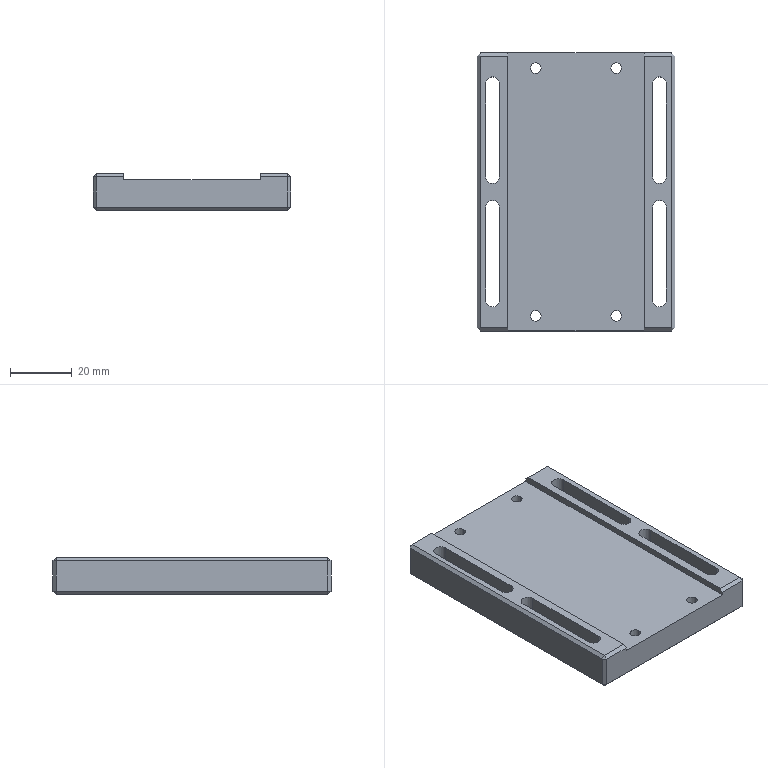Part | STEP file | 07-03 camera fixing plate | 1 solid | 68 faces | box 64 x 90 x 12 mm | volume 52965 mm3 | plane 44 | cylinder 24 | commonest cylinder face diameters 3.4 x8 4.5 x8 6.5 x8